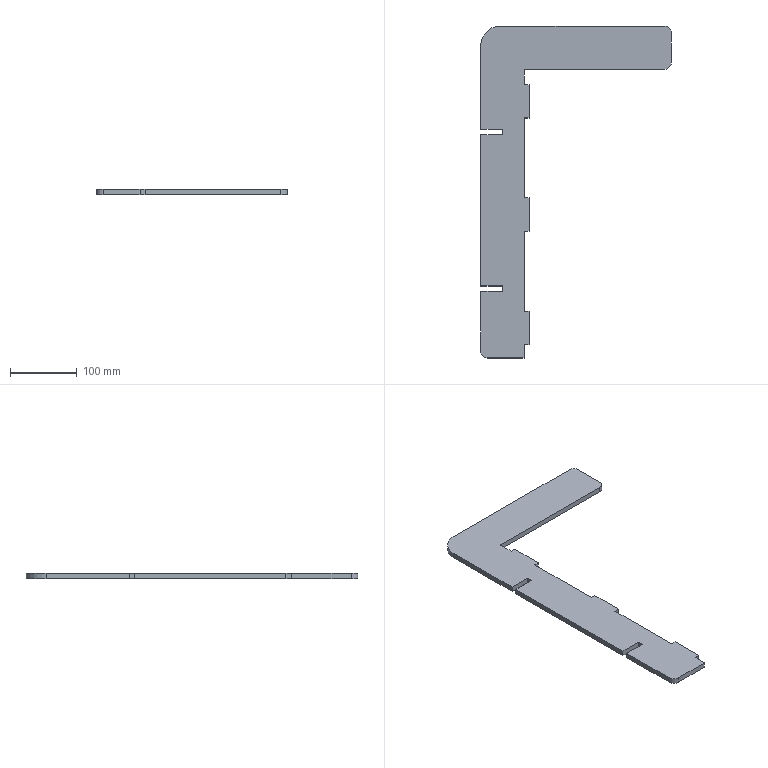Part | SolidWorks | features FlatPattern 1, SMBaseFlange 1, SheetMetal 1 | 1 solid | 33 faces | box 286 x 498 x 8 mm | volume 376603 mm3 | plane 28 | cylinder 5 | commonest cylinder face diameters 20 x3 4 x1 60 x1
STEP:
#1=CARTESIAN_POINT('',(350.505,-222.753,0.));
#2=VERTEX_POINT('',#1);
#3=CARTESIAN_POINT('',(350.505,-202.753,0.));
#4=VERTEX_POINT('',#3);
#5=CARTESIAN_POINT('',(350.505,-222.753,0.));
#6=DIRECTION('',(0.,1.,0.));
#7=VECTOR('',#6,1000.);
#8=LINE('',#5,#7);
#9=EDGE_CURVE('',#2,#4,#8,.T.);
#10=ORIENTED_EDGE('',*,*,#9,.F.);
#11=CARTESIAN_POINT('',(350.505,-222.753,-8.));
#12=VERTEX_POINT('',#11);
#13=CARTESIAN_POINT('',(350.505,-222.753,-8.));
#14=DIRECTION('',(0.,0.,1.));
#15=VECTOR('',#14,1000.);
#16=LINE('',#13,#15);
#17=EDGE_CURVE('',#12,#2,#16,.T.);
#18=ORIENTED_EDGE('',*,*,#17,.F.);
#19=CARTESIAN_POINT('',(350.505,-202.753,-8.));
#20=VERTEX_POINT('',#19);
#21=CARTESIAN_POINT('',(350.505,-222.753,-8.));
#22=DIRECTION('',(0.,1.,0.));
#23=VECTOR('',#22,1000.);
#24=LINE('',#21,#23);
#25=EDGE_CURVE('',#12,#20,#24,.T.);
#26=ORIENTED_EDGE('',*,*,#25,.T.);
#27=CARTESIAN_POINT('',(350.505,-202.753,-8.));
#28=DIRECTION('',(0.,0.,1.));
#29=VECTOR('',#28,1000.);
#30=LINE('',#27,#29);
#31=EDGE_CURVE('',#20,#4,#30,.T.);
#32=ORIENTED_EDGE('',*,*,#31,.T.);
#33=EDGE_LOOP('',(#10,#18,#26,#32));
#34=FACE_OUTER_BOUND('',#33,.T.);
#35=CARTESIAN_POINT('',(350.505,-222.753,-8.));
#36=DIRECTION('',(1.,0.,0.));
#37=DIRECTION('',(0.,0.,-1.));
#38=AXIS2_PLACEMENT_3D('',#35,#36,#37);
#39=PLANE('',#38);
#40=ADVANCED_FACE('',(#34),#39,.T.);
#41=CARTESIAN_POINT('',(295.505,-222.753,0.));
#42=VERTEX_POINT('',#41);
#43=CARTESIAN_POINT('',(295.505,-222.753,0.));
#44=DIRECTION('',(1.,0.,0.));
#45=VECTOR('',#44,1000.);
#46=LINE('',#43,#45);
#47=EDGE_CURVE('',#42,#2,#46,.T.);
#48=ORIENTED_EDGE('',*,*,#47,.F.);
#49=CARTESIAN_POINT('',(295.505,-222.753,-8.));
#50=VERTEX_POINT('',#49);
#51=CARTESIAN_POINT('',(295.505,-222.753,-8.));
#52=DIRECTION('',(0.,0.,1.));
#53=VECTOR('',#52,1000.);
#54=LINE('',#51,#53);
#55=EDGE_CURVE('',#50,#42,#54,.T.);
#56=ORIENTED_EDGE('',*,*,#55,.F.);
#57=CARTESIAN_POINT('',(295.505,-222.753,-8.));
#58=DIRECTION('',(1.,0.,0.));
#59=VECTOR('',#58,1000.);
#60=LINE('',#57,#59);
#61=EDGE_CURVE('',#50,#12,#60,.T.);
#62=ORIENTED_EDGE('',*,*,#61,.T.);
#63=ORIENTED_EDGE('',*,*,#17,.T.);
#64=EDGE_LOOP('',(#48,#56,#62,#63));
#65=FACE_OUTER_BOUND('',#64,.T.);
#66=CARTESIAN_POINT('',(295.505,-222.753,-8.));
#67=DIRECTION('',(0.,-1.,0.));
#68=DIRECTION('',(0.,0.,-1.));
#69=AXIS2_PLACEMENT_3D('',#66,#67,#68);
#70=PLANE('',#69);
#71=ADVANCED_FACE('',(#65),#70,.T.);
#72=CARTESIAN_POINT('',(285.505,-212.753,0.));
#73=VERTEX_POINT('',#72);
#74=CARTESIAN_POINT('',(295.505,-212.753,0.));
#75=DIRECTION('',(0.,0.,1.));
#76=DIRECTION('',(1.,0.,0.));
#77=AXIS2_PLACEMENT_3D('',#74,#75,#76);
#78=CIRCLE('',#77,10.);
#79=EDGE_CURVE('',#73,#42,#78,.T.);
#80=ORIENTED_EDGE('',*,*,#79,.F.);
#81=CARTESIAN_POINT('',(285.505,-212.753,-8.));
#82=VERTEX_POINT('',#81);
#83=CARTESIAN_POINT('',(285.505,-212.753,-8.));
#84=DIRECTION('',(0.,0.,1.));
#85=VECTOR('',#84,1000.);
#86=LINE('',#83,#85);
#87=EDGE_CURVE('',#82,#73,#86,.T.);
#88=ORIENTED_EDGE('',*,*,#87,.F.);
#89=CARTESIAN_POINT('',(295.505,-212.753,-8.));
#90=DIRECTION('',(0.,0.,1.));
#91=DIRECTION('',(1.,0.,0.));
#92=AXIS2_PLACEMENT_3D('',#89,#90,#91);
#93=CIRCLE('',#92,10.);
#94=EDGE_CURVE('',#82,#50,#93,.T.);
#95=ORIENTED_EDGE('',*,*,#94,.T.);
#96=ORIENTED_EDGE('',*,*,#55,.T.);
#97=EDGE_LOOP('',(#80,#88,#95,#96));
#98=FACE_OUTER_BOUND('',#97,.T.);
#99=CARTESIAN_POINT('',(295.505,-212.753,-8.));
#100=DIRECTION('',(0.,0.,1.));
#101=DIRECTION('',(1.,0.,0.));
#102=AXIS2_PLACEMENT_3D('',#99,#100,#101);
#103=CYLINDRICAL_SURFACE('',#102,10.);
#104=ADVANCED_FACE('',(#98),#103,.T.);
#105=CARTESIAN_POINT('',(285.505,-122.753,0.));
#106=VERTEX_POINT('',#105);
#107=CARTESIAN_POINT('',(285.505,-122.753,0.));
#108=DIRECTION('',(0.,-1.,0.));
#109=VECTOR('',#108,1000.);
#110=LINE('',#107,#109);
#111=EDGE_CURVE('',#106,#73,#110,.T.);
#112=ORIENTED_EDGE('',*,*,#111,.F.);
#113=CARTESIAN_POINT('',(285.505,-122.753,-8.));
#114=VERTEX_POINT('',#113);
#115=CARTESIAN_POINT('',(285.505,-122.753,-8.));
#116=DIRECTION('',(0.,0.,1.));
#117=VECTOR('',#116,1000.);
#118=LINE('',#115,#117);
#119=EDGE_CURVE('',#114,#106,#118,.T.);
#120=ORIENTED_EDGE('',*,*,#119,.F.);
#121=CARTESIAN_POINT('',(285.505,-122.753,-8.));
#122=DIRECTION('',(0.,-1.,0.));
#123=VECTOR('',#122,1000.);
#124=LINE('',#121,#123);
#125=EDGE_CURVE('',#114,#82,#124,.T.);
#126=ORIENTED_EDGE('',*,*,#125,.T.);
#127=ORIENTED_EDGE('',*,*,#87,.T.);
#128=EDGE_LOOP('',(#112,#120,#126,#127));
#129=FACE_OUTER_BOUND('',#128,.T.);
#130=CARTESIAN_POINT('',(285.505,-122.753,-8.));
#131=DIRECTION('',(-1.,0.,0.));
#132=DIRECTION('',(0.,-1.,0.));
#133=AXIS2_PLACEMENT_3D('',#130,#131,#132);
#134=PLANE('',#133);
#135=ADVANCED_FACE('',(#129),#134,.T.);
#136=CARTESIAN_POINT('',(318.505,-122.753,0.));
#137=VERTEX_POINT('',#136);
#138=CARTESIAN_POINT('',(318.505,-122.753,0.));
#139=DIRECTION('',(-1.,0.,0.));
#140=VECTOR('',#139,1000.);
#141=LINE('',#138,#140);
#142=EDGE_CURVE('',#137,#106,#141,.T.);
#143=ORIENTED_EDGE('',*,*,#142,.F.);
#144=CARTESIAN_POINT('',(318.505,-122.753,-8.));
#145=VERTEX_POINT('',#144);
#146=CARTESIAN_POINT('',(318.505,-122.753,-8.));
#147=DIRECTION('',(0.,0.,1.));
#148=VECTOR('',#147,1000.);
#149=LINE('',#146,#148);
#150=EDGE_CURVE('',#145,#137,#149,.T.);
#151=ORIENTED_EDGE('',*,*,#150,.F.);
#152=CARTESIAN_POINT('',(318.505,-122.753,-8.));
#153=DIRECTION('',(-1.,0.,0.));
#154=VECTOR('',#153,1000.);
#155=LINE('',#152,#154);
#156=EDGE_CURVE('',#145,#114,#155,.T.);
#157=ORIENTED_EDGE('',*,*,#156,.T.);
#158=ORIENTED_EDGE('',*,*,#119,.T.);
#159=EDGE_LOOP('',(#143,#151,#157,#158));
#160=FACE_OUTER_BOUND('',#159,.T.);
#161=CARTESIAN_POINT('',(318.505,-122.753,-8.));
#162=DIRECTION('',(0.,1.,0.));
#163=DIRECTION('',(-1.,0.,0.));
#164=AXIS2_PLACEMENT_3D('',#161,#162,#163);
#165=PLANE('',#164);
#166=ADVANCED_FACE('',(#160),#165,.T.);
#167=CARTESIAN_POINT('',(318.505,-114.753,0.));
#168=VERTEX_POINT('',#167);
#169=CARTESIAN_POINT('',(318.505,-114.753,0.));
#170=DIRECTION('',(0.,-1.,0.));
#171=VECTOR('',#170,1000.);
#172=LINE('',#169,#171);
#173=EDGE_CURVE('',#168,#137,#172,.T.);
#174=ORIENTED_EDGE('',*,*,#173,.F.);
#175=CARTESIAN_POINT('',(318.505,-114.753,-8.));
#176=VERTEX_POINT('',#175);
#177=CARTESIAN_POINT('',(318.505,-114.753,-8.));
#178=DIRECTION('',(0.,0.,1.));
#179=VECTOR('',#178,1000.);
#180=LINE('',#177,#179);
#181=EDGE_CURVE('',#176,#168,#180,.T.);
#182=ORIENTED_EDGE('',*,*,#181,.F.);
#183=CARTESIAN_POINT('',(318.505,-114.753,-8.));
#184=DIRECTION('',(0.,-1.,0.));
#185=VECTOR('',#184,1000.);
#186=LINE('',#183,#185);
#187=EDGE_CURVE('',#176,#145,#186,.T.);
#188=ORIENTED_EDGE('',*,*,#187,.T.);
#189=ORIENTED_EDGE('',*,*,#150,.T.);
#190=EDGE_LOOP('',(#174,#182,#188,#189));
#191=FACE_OUTER_BOUND('',#190,.T.);
#192=CARTESIAN_POINT('',(318.505,-114.753,-8.));
#193=DIRECTION('',(-1.,0.,0.));
#194=DIRECTION('',(0.,0.,1.));
#195=AXIS2_PLACEMENT_3D('',#192,#193,#194);
#196=PLANE('',#195);
#197=ADVANCED_FACE('',(#191),#196,.T.);
#198=CARTESIAN_POINT('',(285.505,-114.753,0.));
#199=VERTEX_POINT('',#198);
#200=CARTESIAN_POINT('',(285.505,-114.753,0.));
#201=DIRECTION('',(1.,0.,0.));
#202=VECTOR('',#201,1000.);
#203=LINE('',#200,#202);
#204=EDGE_CURVE('',#199,#168,#203,.T.);
#205=ORIENTED_EDGE('',*,*,#204,.F.);
#206=CARTESIAN_POINT('',(285.505,-114.753,-8.));
#207=VERTEX_POINT('',#206);
#208=CARTESIAN_POINT('',(285.505,-114.753,-8.));
#209=DIRECTION('',(0.,0.,1.));
#210=VECTOR('',#209,1000.);
#211=LINE('',#208,#210);
#212=EDGE_CURVE('',#207,#199,#211,.T.);
#213=ORIENTED_EDGE('',*,*,#212,.F.);
#214=CARTESIAN_POINT('',(285.505,-114.753,-8.));
#215=DIRECTION('',(1.,0.,0.));
#216=VECTOR('',#215,1000.);
#217=LINE('',#214,#216);
#218=EDGE_CURVE('',#207,#176,#217,.T.);
#219=ORIENTED_EDGE('',*,*,#218,.T.);
#220=ORIENTED_EDGE('',*,*,#181,.T.);
#221=EDGE_LOOP('',(#205,#213,#219,#220));
#222=FACE_OUTER_BOUND('',#221,.T.);
#223=CARTESIAN_POINT('',(285.505,-114.753,-8.));
#224=DIRECTION('',(0.,-1.,0.));
#225=DIRECTION('',(1.,0.,0.));
#226=AXIS2_PLACEMENT_3D('',#223,#224,#225);
#227=PLANE('',#226);
#228=ADVANCED_FACE('',(#222),#227,.T.);
#229=CARTESIAN_POINT('',(285.505,112.247,0.));
#230=VERTEX_POINT('',#229);
#231=CARTESIAN_POINT('',(285.505,112.247,0.));
#232=DIRECTION('',(0.,-1.,0.));
#233=VECTOR('',#232,1000.);
#234=LINE('',#231,#233);
#235=EDGE_CURVE('',#230,#199,#234,.T.);
#236=ORIENTED_EDGE('',*,*,#235,.F.);
#237=CARTESIAN_POINT('',(285.505,112.247,-8.));
#238=VERTEX_POINT('',#237);
#239=CARTESIAN_POINT('',(285.505,112.247,-8.));
#240=DIRECTION('',(0.,0.,1.));
#241=VECTOR('',#240,1000.);
#242=LINE('',#239,#241);
#243=EDGE_CURVE('',#238,#230,#242,.T.);
#244=ORIENTED_EDGE('',*,*,#243,.F.);
#245=CARTESIAN_POINT('',(285.505,112.247,-8.));
#246=DIRECTION('',(0.,-1.,0.));
#247=VECTOR('',#246,1000.);
#248=LINE('',#245,#247);
#249=EDGE_CURVE('',#238,#207,#248,.T.);
#250=ORIENTED_EDGE('',*,*,#249,.T.);
#251=ORIENTED_EDGE('',*,*,#212,.T.);
#252=EDGE_LOOP('',(#236,#244,#250,#251));
#253=FACE_OUTER_BOUND('',#252,.T.);
#254=CARTESIAN_POINT('',(285.505,112.247,-8.));
#255=DIRECTION('',(-1.,0.,0.));
#256=DIRECTION('',(0.,-1.,0.));
#257=AXIS2_PLACEMENT_3D('',#254,#255,#256);
#258=PLANE('',#257);
#259=ADVANCED_FACE('',(#253),#258,.T.);
#260=CARTESIAN_POINT('',(318.505,112.247,0.));
#261=VERTEX_POINT('',#260);
#262=CARTESIAN_POINT('',(318.505,112.247,0.));
#263=DIRECTION('',(-1.,0.,0.));
#264=VECTOR('',#263,1000.);
#265=LINE('',#262,#264);
#266=EDGE_CURVE('',#261,#230,#265,.T.);
#267=ORIENTED_EDGE('',*,*,#266,.F.);
#268=CARTESIAN_POINT('',(318.505,112.247,-8.));
#269=VERTEX_POINT('',#268);
#270=CARTESIAN_POINT('',(318.505,112.247,-8.));
#271=DIRECTION('',(0.,0.,1.));
#272=VECTOR('',#271,1000.);
#273=LINE('',#270,#272);
#274=EDGE_CURVE('',#269,#261,#273,.T.);
#275=ORIENTED_EDGE('',*,*,#274,.F.);
#276=CARTESIAN_POINT('',(318.505,112.247,-8.));
#277=DIRECTION('',(-1.,0.,0.));
#278=VECTOR('',#277,1000.);
#279=LINE('',#276,#278);
#280=EDGE_CURVE('',#269,#238,#279,.T.);
#281=ORIENTED_EDGE('',*,*,#280,.T.);
#282=ORIENTED_EDGE('',*,*,#243,.T.);
#283=EDGE_LOOP('',(#267,#275,#281,#282));
#284=FACE_OUTER_BOUND('',#283,.T.);
#285=CARTESIAN_POINT('',(318.505,112.247,-8.));
#286=DIRECTION('',(0.,1.,0.));
#287=DIRECTION('',(-1.,0.,0.));
#288=AXIS2_PLACEMENT_3D('',#285,#286,#287);
#289=PLANE('',#288);
#290=ADVANCED_FACE('',(#284),#289,.T.);
#291=CARTESIAN_POINT('',(318.505,120.247,0.));
#292=VERTEX_POINT('',#291);
#293=CARTESIAN_POINT('',(318.505,120.247,0.));
#294=DIRECTION('',(0.,-1.,0.));
#295=VECTOR('',#294,1000.);
#296=LINE('',#293,#295);
#297=EDGE_CURVE('',#292,#261,#296,.T.);
#298=ORIENTED_EDGE('',*,*,#297,.F.);
#299=CARTESIAN_POINT('',(318.505,120.247,-8.));
#300=VERTEX_POINT('',#299);
#301=CARTESIAN_POINT('',(318.505,120.247,-8.));
#302=DIRECTION('',(0.,0.,1.));
#303=VECTOR('',#302,1000.);
#304=LINE('',#301,#303);
#305=EDGE_CURVE('',#300,#292,#304,.T.);
#306=ORIENTED_EDGE('',*,*,#305,.F.);
#307=CARTESIAN_POINT('',(318.505,120.247,-8.));
#308=DIRECTION('',(0.,-1.,0.));
#309=VECTOR('',#308,1000.);
#310=LINE('',#307,#309);
#311=EDGE_CURVE('',#300,#269,#310,.T.);
#312=ORIENTED_EDGE('',*,*,#311,.T.);
#313=ORIENTED_EDGE('',*,*,#274,.T.);
#314=EDGE_LOOP('',(#298,#306,#312,#313));
#315=FACE_OUTER_BOUND('',#314,.T.);
#316=CARTESIAN_POINT('',(318.505,120.247,-8.));
#317=DIRECTION('',(-1.,0.,0.));
#318=DIRECTION('',(0.,0.,1.));
#319=AXIS2_PLACEMENT_3D('',#316,#317,#318);
#320=PLANE('',#319);
#321=ADVANCED_FACE('',(#315),#320,.T.);
#322=CARTESIAN_POINT('',(285.505,120.247,0.));
#323=VERTEX_POINT('',#322);
#324=CARTESIAN_POINT('',(318.505,120.247,0.));
#325=DIRECTION('',(1.,0.,0.));
#326=VECTOR('',#325,1000.);
#327=LINE('',#324,#326);
#328=EDGE_CURVE('',#323,#292,#327,.T.);
#329=ORIENTED_EDGE('',*,*,#328,.F.);
#330=CARTESIAN_POINT('',(285.505,120.247,-8.));
#331=VERTEX_POINT('',#330);
#332=CARTESIAN_POINT('',(285.505,120.247,-8.));
#333=DIRECTION('',(0.,0.,1.));
#334=VECTOR('',#333,1000.);
#335=LINE('',#332,#334);
#336=EDGE_CURVE('',#331,#323,#335,.T.);
#337=ORIENTED_EDGE('',*,*,#336,.F.);
#338=CARTESIAN_POINT('',(318.505,120.247,-8.));
#339=DIRECTION('',(1.,0.,0.));
#340=VECTOR('',#339,1000.);
#341=LINE('',#338,#340);
#342=EDGE_CURVE('',#331,#300,#341,.T.);
#343=ORIENTED_EDGE('',*,*,#342,.T.);
#344=ORIENTED_EDGE('',*,*,#305,.T.);
#345=EDGE_LOOP('',(#329,#337,#343,#344));
#346=FACE_OUTER_BOUND('',#345,.T.);
#347=CARTESIAN_POINT('',(318.505,120.247,-8.));
#348=DIRECTION('',(0.,-1.,0.));
#349=DIRECTION('',(1.,0.,0.));
#350=AXIS2_PLACEMENT_3D('',#347,#348,#349);
#351=PLANE('',#350);
#352=ADVANCED_FACE('',(#346),#351,.T.);
#353=CARTESIAN_POINT('',(285.505,245.247,0.));
#354=VERTEX_POINT('',#353);
#355=CARTESIAN_POINT('',(285.505,245.247,0.));
#356=DIRECTION('',(0.,-1.,0.));
#357=VECTOR('',#356,1000.);
#358=LINE('',#355,#357);
#359=EDGE_CURVE('',#354,#323,#358,.T.);
#360=ORIENTED_EDGE('',*,*,#359,.F.);
#361=CARTESIAN_POINT('',(285.505,245.247,-8.));
#362=VERTEX_POINT('',#361);
#363=CARTESIAN_POINT('',(285.505,245.247,-8.));
#364=DIRECTION('',(0.,0.,1.));
#365=VECTOR('',#364,1000.);
#366=LINE('',#363,#365);
#367=EDGE_CURVE('',#362,#354,#366,.T.);
#368=ORIENTED_EDGE('',*,*,#367,.F.);
#369=CARTESIAN_POINT('',(285.505,245.247,-8.));
#370=DIRECTION('',(0.,-1.,0.));
#371=VECTOR('',#370,1000.);
#372=LINE('',#369,#371);
#373=EDGE_CURVE('',#362,#331,#372,.T.);
#374=ORIENTED_EDGE('',*,*,#373,.T.);
#375=ORIENTED_EDGE('',*,*,#336,.T.);
#376=EDGE_LOOP('',(#360,#368,#374,#375));
#377=FACE_OUTER_BOUND('',#376,.T.);
#378=CARTESIAN_POINT('',(285.505,245.247,-8.));
#379=DIRECTION('',(-1.,0.,0.));
#380=DIRECTION('',(0.,-1.,0.));
#381=AXIS2_PLACEMENT_3D('',#378,#379,#380);
#382=PLANE('',#381);
#383=ADVANCED_FACE('',(#377),#382,.T.);
#384=CARTESIAN_POINT('',(315.505,275.247,0.));
#385=VERTEX_POINT('',#384);
#386=CARTESIAN_POINT('',(315.505,245.247,0.));
#387=DIRECTION('',(0.,0.,1.));
#388=DIRECTION('',(1.,0.,0.));
#389=AXIS2_PLACEMENT_3D('',#386,#387,#388);
#390=CIRCLE('',#389,30.);
#391=EDGE_CURVE('',#385,#354,#390,.T.);
#392=ORIENTED_EDGE('',*,*,#391,.F.);
#393=CARTESIAN_POINT('',(315.505,275.247,-8.));
#394=VERTEX_POINT('',#393);
#395=CARTESIAN_POINT('',(315.505,275.247,-8.));
#396=DIRECTION('',(0.,0.,1.));
#397=VECTOR('',#396,1000.);
#398=LINE('',#395,#397);
#399=EDGE_CURVE('',#394,#385,#398,.T.);
#400=ORIENTED_EDGE('',*,*,#399,.F.);
#401=CARTESIAN_POINT('',(315.505,245.247,-8.));
#402=DIRECTION('',(0.,0.,1.));
#403=DIRECTION('',(1.,0.,0.));
#404=AXIS2_PLACEMENT_3D('',#401,#402,#403);
#405=CIRCLE('',#404,30.);
#406=EDGE_CURVE('',#394,#362,#405,.T.);
#407=ORIENTED_EDGE('',*,*,#406,.T.);
#408=ORIENTED_EDGE('',*,*,#367,.T.);
#409=EDGE_LOOP('',(#392,#400,#407,#408));
#410=FACE_OUTER_BOUND('',#409,.T.);
#411=CARTESIAN_POINT('',(315.505,245.247,-8.));
#412=DIRECTION('',(0.,0.,1.));
#413=DIRECTION('',(1.,0.,0.));
#414=AXIS2_PLACEMENT_3D('',#411,#412,#413);
#415=CYLINDRICAL_SURFACE('',#414,30.);
#416=ADVANCED_FACE('',(#410),#415,.T.);
#417=CARTESIAN_POINT('',(561.505,275.247,0.));
#418=VERTEX_POINT('',#417);
#419=CARTESIAN_POINT('',(561.505,275.247,0.));
#420=DIRECTION('',(-1.,0.,0.));
#421=VECTOR('',#420,1000.);
#422=LINE('',#419,#421);
#423=EDGE_CURVE('',#418,#385,#422,.T.);
#424=ORIENTED_EDGE('',*,*,#423,.F.);
#425=CARTESIAN_POINT('',(561.505,275.247,-8.));
#426=VERTEX_POINT('',#425);
#427=CARTESIAN_POINT('',(561.505,275.247,-8.));
#428=DIRECTION('',(0.,0.,1.));
#429=VECTOR('',#428,1000.);
#430=LINE('',#427,#429);
#431=EDGE_CURVE('',#426,#418,#430,.T.);
#432=ORIENTED_EDGE('',*,*,#431,.F.);
#433=CARTESIAN_POINT('',(561.505,275.247,-8.));
#434=DIRECTION('',(-1.,0.,0.));
#435=VECTOR('',#434,1000.);
#436=LINE('',#433,#435);
#437=EDGE_CURVE('',#426,#394,#436,.T.);
#438=ORIENTED_EDGE('',*,*,#437,.T.);
#439=ORIENTED_EDGE('',*,*,#399,.T.);
#440=EDGE_LOOP('',(#424,#432,#438,#439));
#441=FACE_OUTER_BOUND('',#440,.T.);
#442=CARTESIAN_POINT('',(561.505,275.247,-8.));
#443=DIRECTION('',(0.,1.,0.));
#444=DIRECTION('',(-1.,0.,0.));
#445=AXIS2_PLACEMENT_3D('',#442,#443,#444);
#446=PLANE('',#445);
#447=ADVANCED_FACE('',(#441),#446,.T.);
#448=CARTESIAN_POINT('',(571.505,265.247,0.));
#449=VERTEX_POINT('',#448);
#450=CARTESIAN_POINT('',(561.505,265.247,0.));
#451=DIRECTION('',(0.,0.,1.));
#452=DIRECTION('',(1.,0.,0.));
#453=AXIS2_PLACEMENT_3D('',#450,#451,#452);
#454=CIRCLE('',#453,10.);
#455=EDGE_CURVE('',#449,#418,#454,.T.);
#456=ORIENTED_EDGE('',*,*,#455,.F.);
#457=CARTESIAN_POINT('',(571.505,265.247,-8.));
#458=VERTEX_POINT('',#457);
#459=CARTESIAN_POINT('',(571.505,265.247,-8.));
#460=DIRECTION('',(0.,0.,1.));
#461=VECTOR('',#460,1000.);
#462=LINE('',#459,#461);
#463=EDGE_CURVE('',#458,#449,#462,.T.);
#464=ORIENTED_EDGE('',*,*,#463,.F.);
#465=CARTESIAN_POINT('',(561.505,265.247,-8.));
#466=DIRECTION('',(0.,0.,1.));
#467=DIRECTION('',(1.,0.,0.));
#468=AXIS2_PLACEMENT_3D('',#465,#466,#467);
#469=CIRCLE('',#468,10.);
#470=EDGE_CURVE('',#458,#426,#469,.T.);
#471=ORIENTED_EDGE('',*,*,#470,.T.);
#472=ORIENTED_EDGE('',*,*,#431,.T.);
#473=EDGE_LOOP('',(#456,#464,#471,#472));
#474=FACE_OUTER_BOUND('',#473,.T.);
#475=CARTESIAN_POINT('',(561.505,265.247,-8.));
#476=DIRECTION('',(0.,0.,1.));
#477=DIRECTION('',(1.,0.,0.));
#478=AXIS2_PLACEMENT_3D('',#475,#476,#477);
#479=CYLINDRICAL_SURFACE('',#478,10.);
#480=ADVANCED_FACE('',(#474),#479,.T.);
#481=CARTESIAN_POINT('',(571.505,220.247,0.));
#482=VERTEX_POINT('',#481);
#483=CARTESIAN_POINT('',(571.505,220.247,0.));
#484=DIRECTION('',(0.,1.,0.));
#485=VECTOR('',#484,1000.);
#486=LINE('',#483,#485);
#487=EDGE_CURVE('',#482,#449,#486,.T.);
#488=ORIENTED_EDGE('',*,*,#487,.F.);
#489=CARTESIAN_POINT('',(571.505,220.247,-8.));
#490=VERTEX_POINT('',#489);
#491=CARTESIAN_POINT('',(571.505,220.247,-8.));
#492=DIRECTION('',(0.,0.,1.));
#493=VECTOR('',#492,1000.);
#494=LINE('',#491,#493);
#495=EDGE_CURVE('',#490,#482,#494,.T.);
#496=ORIENTED_EDGE('',*,*,#495,.F.);
#497=CARTESIAN_POINT('',(571.505,220.247,-8.));
#498=DIRECTION('',(0.,1.,0.));
#499=VECTOR('',#498,1000.);
#500=LINE('',#497,#499);
#501=EDGE_CURVE('',#490,#458,#500,.T.);
#502=ORIENTED_EDGE('',*,*,#501,.T.);
#503=ORIENTED_EDGE('',*,*,#463,.T.);
#504=EDGE_LOOP('',(#488,#496,#502,#503));
#505=FACE_OUTER_BOUND('',#504,.T.);
#506=CARTESIAN_POINT('',(571.505,220.247,-8.));
#507=DIRECTION('',(1.,0.,0.));
#508=DIRECTION('',(0.,1.,0.));
#509=AXIS2_PLACEMENT_3D('',#506,#507,#508);
#510=PLANE('',#509);
#511=ADVANCED_FACE('',(#505),#510,.T.);
#512=CARTESIAN_POINT('',(561.505,210.247,0.));
#513=VERTEX_POINT('',#512);
#514=CARTESIAN_POINT('',(561.505,220.247,0.));
#515=DIRECTION('',(0.,0.,1.));
#516=DIRECTION('',(1.,0.,0.));
#517=AXIS2_PLACEMENT_3D('',#514,#515,#516);
#518=CIRCLE('',#517,10.);
#519=EDGE_CURVE('',#513,#482,#518,.T.);
#520=ORIENTED_EDGE('',*,*,#519,.F.);
#521=CARTESIAN_POINT('',(561.505,210.247,-8.));
#522=VERTEX_POINT('',#521);
#523=CARTESIAN_POINT('',(561.505,210.247,-8.));
#524=DIRECTION('',(0.,0.,1.));
#525=VECTOR('',#524,1000.);
#526=LINE('',#523,#525);
#527=EDGE_CURVE('',#522,#513,#526,.T.);
#528=ORIENTED_EDGE('',*,*,#527,.F.);
#529=CARTESIAN_POINT('',(561.505,220.247,-8.));
#530=DIRECTION('',(0.,0.,1.));
#531=DIRECTION('',(1.,0.,0.));
#532=AXIS2_PLACEMENT_3D('',#529,#530,#531);
#533=CIRCLE('',#532,10.);
#534=EDGE_CURVE('',#522,#490,#533,.T.);
#535=ORIENTED_EDGE('',*,*,#534,.T.);
#536=ORIENTED_EDGE('',*,*,#495,.T.);
#537=EDGE_LOOP('',(#520,#528,#535,#536));
#538=FACE_OUTER_BOUND('',#537,.T.);
#539=CARTESIAN_POINT('',(561.505,220.247,-8.));
#540=DIRECTION('',(0.,0.,1.));
#541=DIRECTION('',(1.,0.,0.));
#542=AXIS2_PLACEMENT_3D('',#539,#540,#541);
#543=CYLINDRICAL_SURFACE('',#542,10.);
#544=ADVANCED_FACE('',(#538),#543,.T.);
#545=CARTESIAN_POINT('',(352.505,210.247,0.));
#546=VERTEX_POINT('',#545);
#547=CARTESIAN_POINT('',(352.505,210.247,0.));
#548=DIRECTION('',(1.,0.,0.));
#549=VECTOR('',#548,1000.);
#550=LINE('',#547,#549);
#551=EDGE_CURVE('',#546,#513,#550,.T.);
#552=ORIENTED_EDGE('',*,*,#551,.F.);
#553=CARTESIAN_POINT('',(352.505,210.247,-8.));
#554=VERTEX_POINT('',#553);
#555=CARTESIAN_POINT('',(352.505,210.247,-8.));
#556=DIRECTION('',(0.,0.,1.));
#557=VECTOR('',#556,1000.);
#558=LINE('',#555,#557);
#559=EDGE_CURVE('',#554,#546,#558,.T.);
#560=ORIENTED_EDGE('',*,*,#559,.F.);
#561=CARTESIAN_POINT('',(352.505,210.247,-8.));
#562=DIRECTION('',(1.,0.,0.));
#563=VECTOR('',#562,1000.);
#564=LINE('',#561,#563);
#565=EDGE_CURVE('',#554,#522,#564,.T.);
#566=ORIENTED_EDGE('',*,*,#565,.T.);
#567=ORIENTED_EDGE('',*,*,#527,.T.);
#568=EDGE_LOOP('',(#552,#560,#566,#567));
#569=FACE_OUTER_BOUND('',#568,.T.);
#570=CARTESIAN_POINT('',(352.505,210.247,-8.));
#571=DIRECTION('',(0.,-1.,0.));
#572=DIRECTION('',(0.,0.,-1.));
#573=AXIS2_PLACEMENT_3D('',#570,#571,#572);
#574=PLANE('',#573);
#575=ADVANCED_FACE('',(#569),#574,.T.);
#576=CARTESIAN_POINT('',(350.505,208.247,0.));
#577=VERTEX_POINT('',#576);
#578=CARTESIAN_POINT('',(352.505,208.247,0.));
#579=DIRECTION('',(0.,0.,-1.));
#580=DIRECTION('',(-1.,0.,0.));
#581=AXIS2_PLACEMENT_3D('',#578,#579,#580);
#582=CIRCLE('',#581,2.);
#583=EDGE_CURVE('',#577,#546,#582,.T.);
#584=ORIENTED_EDGE('',*,*,#583,.F.);
#585=CARTESIAN_POINT('',(350.505,208.247,-8.));
#586=VERTEX_POINT('',#585);
#587=CARTESIAN_POINT('',(350.505,208.247,-8.));
#588=DIRECTION('',(0.,0.,1.));
#589=VECTOR('',#588,1000.);
#590=LINE('',#587,#589);
#591=EDGE_CURVE('',#586,#577,#590,.T.);
#592=ORIENTED_EDGE('',*,*,#591,.F.);
#593=CARTESIAN_POINT('',(352.505,208.247,-8.));
#594=DIRECTION('',(0.,0.,-1.));
#595=DIRECTION('',(-1.,0.,0.));
#596=AXIS2_PLACEMENT_3D('',#593,#594,#595);
#597=CIRCLE('',#596,2.);
#598=EDGE_CURVE('',#586,#554,#597,.T.);
#599=ORIENTED_EDGE('',*,*,#598,.T.);
#600=ORIENTED_EDGE('',*,*,#559,.T.);
#601=EDGE_LOOP('',(#584,#592,#599,#600));
#602=FACE_OUTER_BOUND('',#601,.T.);
#603=CARTESIAN_POINT('',(352.505,208.247,-8.));
#604=DIRECTION('',(0.,0.,1.));
#605=DIRECTION('',(1.,0.,0.));
#606=AXIS2_PLACEMENT_3D('',#603,#604,#605);
#607=CYLINDRICAL_SURFACE('',#606,2.);
#608=ADVANCED_FACE('',(#602),#607,.F.);
#609=CARTESIAN_POINT('',(350.505,187.247,0.));
#610=VERTEX_POINT('',#609);
#611=CARTESIAN_POINT('',(350.505,187.247,0.));
#612=DIRECTION('',(0.,1.,0.));
#613=VECTOR('',#612,1000.);
#614=LINE('',#611,#613);
#615=EDGE_CURVE('',#610,#577,#614,.T.);
#616=ORIENTED_EDGE('',*,*,#615,.F.);
#617=CARTESIAN_POINT('',(350.505,187.247,-8.));
#618=VERTEX_POINT('',#617);
#619=CARTESIAN_POINT('',(350.505,187.247,-8.));
#620=DIRECTION('',(0.,0.,1.));
#621=VECTOR('',#620,1000.);
#622=LINE('',#619,#621);
#623=EDGE_CURVE('',#618,#610,#622,.T.);
#624=ORIENTED_EDGE('',*,*,#623,.F.);
#625=CARTESIAN_POINT('',(350.505,187.247,-8.));
#626=DIRECTION('',(0.,1.,0.));
#627=VECTOR('',#626,1000.);
#628=LINE('',#625,#627);
#629=EDGE_CURVE('',#618,#586,#628,.T.);
#630=ORIENTED_EDGE('',*,*,#629,.T.);
#631=ORIENTED_EDGE('',*,*,#591,.T.);
#632=EDGE_LOOP('',(#616,#624,#630,#631));
#633=FACE_OUTER_BOUND('',#632,.T.);
#634=CARTESIAN_POINT('',(350.505,187.247,-8.));
#635=DIRECTION('',(1.,0.,0.));
#636=DIRECTION('',(0.,1.,0.));
#637=AXIS2_PLACEMENT_3D('',#634,#635,#636);
#638=PLANE('',#637);
#639=ADVANCED_FACE('',(#633),#638,.T.);
#640=CARTESIAN_POINT('',(358.005,187.247,0.));
#641=VERTEX_POINT('',#640);
#642=CARTESIAN_POINT('',(358.005,187.247,0.));
#643=DIRECTION('',(-1.,0.,0.));
#644=VECTOR('',#643,1000.);
#645=LINE('',#642,#644);
#646=EDGE_CURVE('',#641,#610,#645,.T.);
#647=ORIENTED_EDGE('',*,*,#646,.F.);
#648=CARTESIAN_POINT('',(358.005,187.247,-8.));
#649=VERTEX_POINT('',#648);
#650=CARTESIAN_POINT('',(358.005,187.247,-8.));
#651=DIRECTION('',(0.,0.,1.));
#652=VECTOR('',#651,1000.);
#653=LINE('',#650,#652);
#654=EDGE_CURVE('',#649,#641,#653,.T.);
#655=ORIENTED_EDGE('',*,*,#654,.F.);
#656=CARTESIAN_POINT('',(358.005,187.247,-8.));
#657=DIRECTION('',(-1.,0.,0.));
#658=VECTOR('',#657,1000.);
#659=LINE('',#656,#658);
#660=EDGE_CURVE('',#649,#618,#659,.T.);
#661=ORIENTED_EDGE('',*,*,#660,.T.);
#662=ORIENTED_EDGE('',*,*,#623,.T.);
#663=EDGE_LOOP('',(#647,#655,#661,#662));
#664=FACE_OUTER_BOUND('',#663,.T.);
#665=CARTESIAN_POINT('',(358.005,187.247,-8.));
#666=DIRECTION('',(0.,1.,0.));
#667=DIRECTION('',(0.,0.,1.));
#668=AXIS2_PLACEMENT_3D('',#665,#666,#667);
#669=PLANE('',#668);
#670=ADVANCED_FACE('',(#664),#669,.T.);
#671=CARTESIAN_POINT('',(358.005,137.247,0.));
#672=VERTEX_POINT('',#671);
#673=CARTESIAN_POINT('',(358.005,137.247,0.));
#674=DIRECTION('',(0.,1.,0.));
#675=VECTOR('',#674,1000.);
#676=LINE('',#673,#675);
#677=EDGE_CURVE('',#672,#641,#676,.T.);
#678=ORIENTED_EDGE('',*,*,#677,.F.);
#679=CARTESIAN_POINT('',(358.005,137.247,-8.));
#680=VERTEX_POINT('',#679);
#681=CARTESIAN_POINT('',(358.005,137.247,-8.));
#682=DIRECTION('',(0.,0.,1.));
#683=VECTOR('',#682,1000.);
#684=LINE('',#681,#683);
#685=EDGE_CURVE('',#680,#672,#684,.T.);
#686=ORIENTED_EDGE('',*,*,#685,.F.);
#687=CARTESIAN_POINT('',(358.005,137.247,-8.));
#688=DIRECTION('',(0.,1.,0.));
#689=VECTOR('',#688,1000.);
#690=LINE('',#687,#689);
#691=EDGE_CURVE('',#680,#649,#690,.T.);
#692=ORIENTED_EDGE('',*,*,#691,.T.);
#693=ORIENTED_EDGE('',*,*,#654,.T.);
#694=EDGE_LOOP('',(#678,#686,#692,#693));
#695=FACE_OUTER_BOUND('',#694,.T.);
#696=CARTESIAN_POINT('',(358.005,137.247,-8.));
#697=DIRECTION('',(1.,0.,0.));
#698=DIRECTION('',(0.,0.,-1.));
#699=AXIS2_PLACEMENT_3D('',#696,#697,#698);
#700=PLANE('',#699);
#701=ADVANCED_FACE('',(#695),#700,.T.);
#702=CARTESIAN_POINT('',(350.505,137.247,0.));
#703=VERTEX_POINT('',#702);
#704=CARTESIAN_POINT('',(350.505,137.247,0.));
#705=DIRECTION('',(1.,0.,0.));
#706=VECTOR('',#705,1000.);
#707=LINE('',#704,#706);
#708=EDGE_CURVE('',#703,#672,#707,.T.);
#709=ORIENTED_EDGE('',*,*,#708,.F.);
#710=CARTESIAN_POINT('',(350.505,137.247,-8.));
#711=VERTEX_POINT('',#710);
#712=CARTESIAN_POINT('',(350.505,137.247,-8.));
#713=DIRECTION('',(0.,0.,1.));
#714=VECTOR('',#713,1000.);
#715=LINE('',#712,#714);
#716=EDGE_CURVE('',#711,#703,#715,.T.);
#717=ORIENTED_EDGE('',*,*,#716,.F.);
#718=CARTESIAN_POINT('',(350.505,137.247,-8.));
#719=DIRECTION('',(1.,0.,0.));
#720=VECTOR('',#719,1000.);
#721=LINE('',#718,#720);
#722=EDGE_CURVE('',#711,#680,#721,.T.);
#723=ORIENTED_EDGE('',*,*,#722,.T.);
#724=ORIENTED_EDGE('',*,*,#685,.T.);
#725=EDGE_LOOP('',(#709,#717,#723,#724));
#726=FACE_OUTER_BOUND('',#725,.T.);
#727=CARTESIAN_POINT('',(350.505,137.247,-8.));
#728=DIRECTION('',(0.,-1.,0.));
#729=DIRECTION('',(0.,0.,-1.));
#730=AXIS2_PLACEMENT_3D('',#727,#728,#729);
#731=PLANE('',#730);
#732=ADVANCED_FACE('',(#726),#731,.T.);
#733=CARTESIAN_POINT('',(350.505,17.247,0.));
#734=VERTEX_POINT('',#733);
#735=CARTESIAN_POINT('',(350.505,17.247,0.));
#736=DIRECTION('',(0.,1.,0.));
#737=VECTOR('',#736,1000.);
#738=LINE('',#735,#737);
#739=EDGE_CURVE('',#734,#703,#738,.T.);
#740=ORIENTED_EDGE('',*,*,#739,.F.);
#741=CARTESIAN_POINT('',(350.505,17.247,-8.));
#742=VERTEX_POINT('',#741);
#743=CARTESIAN_POINT('',(350.505,17.247,-8.));
#744=DIRECTION('',(0.,0.,1.));
#745=VECTOR('',#744,1000.);
#746=LINE('',#743,#745);
#747=EDGE_CURVE('',#742,#734,#746,.T.);
#748=ORIENTED_EDGE('',*,*,#747,.F.);
#749=CARTESIAN_POINT('',(350.505,17.247,-8.));
#750=DIRECTION('',(0.,1.,0.));
#751=VECTOR('',#750,1000.);
#752=LINE('',#749,#751);
#753=EDGE_CURVE('',#742,#711,#752,.T.);
#754=ORIENTED_EDGE('',*,*,#753,.T.);
#755=ORIENTED_EDGE('',*,*,#716,.T.);
#756=EDGE_LOOP('',(#740,#748,#754,#755));
#757=FACE_OUTER_BOUND('',#756,.T.);
#758=CARTESIAN_POINT('',(350.505,17.247,-8.));
#759=DIRECTION('',(1.,0.,0.));
#760=DIRECTION('',(0.,0.,-1.));
#761=AXIS2_PLACEMENT_3D('',#758,#759,#760);
#762=PLANE('',#761);
#763=ADVANCED_FACE('',(#757),#762,.T.);
#764=CARTESIAN_POINT('',(358.005,17.247,0.));
#765=VERTEX_POINT('',#764);
#766=CARTESIAN_POINT('',(358.005,17.247,0.));
#767=DIRECTION('',(-1.,0.,0.));
#768=VECTOR('',#767,1000.);
#769=LINE('',#766,#768);
#770=EDGE_CURVE('',#765,#734,#769,.T.);
#771=ORIENTED_EDGE('',*,*,#770,.F.);
#772=CARTESIAN_POINT('',(358.005,17.247,-8.));
#773=VERTEX_POINT('',#772);
#774=CARTESIAN_POINT('',(358.005,17.247,-8.));
#775=DIRECTION('',(0.,0.,1.));
#776=VECTOR('',#775,1000.);
#777=LINE('',#774,#776);
#778=EDGE_CURVE('',#773,#765,#777,.T.);
#779=ORIENTED_EDGE('',*,*,#778,.F.);
#780=CARTESIAN_POINT('',(358.005,17.247,-8.));
#781=DIRECTION('',(-1.,0.,0.));
#782=VECTOR('',#781,1000.);
#783=LINE('',#780,#782);
#784=EDGE_CURVE('',#773,#742,#783,.T.);
#785=ORIENTED_EDGE('',*,*,#784,.T.);
#786=ORIENTED_EDGE('',*,*,#747,.T.);
#787=EDGE_LOOP('',(#771,#779,#785,#786));
#788=FACE_OUTER_BOUND('',#787,.T.);
#789=CARTESIAN_POINT('',(358.005,17.247,-8.));
#790=DIRECTION('',(0.,1.,0.));
#791=DIRECTION('',(0.,0.,1.));
#792=AXIS2_PLACEMENT_3D('',#789,#790,#791);
#793=PLANE('',#792);
#794=ADVANCED_FACE('',(#788),#793,.T.);
#795=CARTESIAN_POINT('',(358.005,-32.753,0.));
#796=VERTEX_POINT('',#795);
#797=CARTESIAN_POINT('',(358.005,-32.753,0.));
#798=DIRECTION('',(0.,1.,0.));
#799=VECTOR('',#798,1000.);
#800=LINE('',#797,#799);
#801=EDGE_CURVE('',#796,#765,#800,.T.);
#802=ORIENTED_EDGE('',*,*,#801,.F.);
#803=CARTESIAN_POINT('',(358.005,-32.753,-8.));
#804=VERTEX_POINT('',#803);
#805=CARTESIAN_POINT('',(358.005,-32.753,-8.));
#806=DIRECTION('',(0.,0.,1.));
#807=VECTOR('',#806,1000.);
#808=LINE('',#805,#807);
#809=EDGE_CURVE('',#804,#796,#808,.T.);
#810=ORIENTED_EDGE('',*,*,#809,.F.);
#811=CARTESIAN_POINT('',(358.005,-32.753,-8.));
#812=DIRECTION('',(0.,1.,0.));
#813=VECTOR('',#812,1000.);
#814=LINE('',#811,#813);
#815=EDGE_CURVE('',#804,#773,#814,.T.);
#816=ORIENTED_EDGE('',*,*,#815,.T.);
#817=ORIENTED_EDGE('',*,*,#778,.T.);
#818=EDGE_LOOP('',(#802,#810,#816,#817));
#819=FACE_OUTER_BOUND('',#818,.T.);
#820=CARTESIAN_POINT('',(358.005,-32.753,-8.));
#821=DIRECTION('',(1.,0.,0.));
#822=DIRECTION('',(0.,0.,-1.));
#823=AXIS2_PLACEMENT_3D('',#820,#821,#822);
#824=PLANE('',#823);
#825=ADVANCED_FACE('',(#819),#824,.T.);
#826=CARTESIAN_POINT('',(350.505,-32.753,0.));
#827=VERTEX_POINT('',#826);
#828=CARTESIAN_POINT('',(350.505,-32.753,0.));
#829=DIRECTION('',(1.,0.,0.));
#830=VECTOR('',#829,1000.);
#831=LINE('',#828,#830);
#832=EDGE_CURVE('',#827,#796,#831,.T.);
#833=ORIENTED_EDGE('',*,*,#832,.F.);
#834=CARTESIAN_POINT('',(350.505,-32.753,-8.));
#835=VERTEX_POINT('',#834);
#836=CARTESIAN_POINT('',(350.505,-32.753,-8.));
#837=DIRECTION('',(0.,0.,1.));
#838=VECTOR('',#837,1000.);
#839=LINE('',#836,#838);
#840=EDGE_CURVE('',#835,#827,#839,.T.);
#841=ORIENTED_EDGE('',*,*,#840,.F.);
#842=CARTESIAN_POINT('',(350.505,-32.753,-8.));
#843=DIRECTION('',(1.,0.,0.));
#844=VECTOR('',#843,1000.);
#845=LINE('',#842,#844);
#846=EDGE_CURVE('',#835,#804,#845,.T.);
#847=ORIENTED_EDGE('',*,*,#846,.T.);
#848=ORIENTED_EDGE('',*,*,#809,.T.);
#849=EDGE_LOOP('',(#833,#841,#847,#848));
#850=FACE_OUTER_BOUND('',#849,.T.);
#851=CARTESIAN_POINT('',(350.505,-32.753,-8.));
#852=DIRECTION('',(0.,-1.,0.));
#853=DIRECTION('',(0.,0.,-1.));
#854=AXIS2_PLACEMENT_3D('',#851,#852,#853);
#855=PLANE('',#854);
#856=ADVANCED_FACE('',(#850),#855,.T.);
#857=CARTESIAN_POINT('',(350.505,-152.753,0.));
#858=VERTEX_POINT('',#857);
#859=CARTESIAN_POINT('',(350.505,-152.753,0.));
#860=DIRECTION('',(0.,1.,0.));
#861=VECTOR('',#860,1000.);
#862=LINE('',#859,#861);
#863=EDGE_CURVE('',#858,#827,#862,.T.);
#864=ORIENTED_EDGE('',*,*,#863,.F.);
#865=CARTESIAN_POINT('',(350.505,-152.753,-8.));
#866=VERTEX_POINT('',#865);
#867=CARTESIAN_POINT('',(350.505,-152.753,-8.));
#868=DIRECTION('',(0.,0.,1.));
#869=VECTOR('',#868,1000.);
#870=LINE('',#867,#869);
#871=EDGE_CURVE('',#866,#858,#870,.T.);
#872=ORIENTED_EDGE('',*,*,#871,.F.);
#873=CARTESIAN_POINT('',(350.505,-152.753,-8.));
#874=DIRECTION('',(0.,1.,0.));
#875=VECTOR('',#874,1000.);
#876=LINE('',#873,#875);
#877=EDGE_CURVE('',#866,#835,#876,.T.);
#878=ORIENTED_EDGE('',*,*,#877,.T.);
#879=ORIENTED_EDGE('',*,*,#840,.T.);
#880=EDGE_LOOP('',(#864,#872,#878,#879));
#881=FACE_OUTER_BOUND('',#880,.T.);
#882=CARTESIAN_POINT('',(350.505,-152.753,-8.));
#883=DIRECTION('',(1.,0.,0.));
#884=DIRECTION('',(0.,0.,-1.));
#885=AXIS2_PLACEMENT_3D('',#882,#883,#884);
#886=PLANE('',#885);
#887=ADVANCED_FACE('',(#881),#886,.T.);
#888=CARTESIAN_POINT('',(358.005,-152.753,0.));
#889=VERTEX_POINT('',#888);
#890=CARTESIAN_POINT('',(358.005,-152.753,0.));
#891=DIRECTION('',(-1.,0.,0.));
#892=VECTOR('',#891,1000.);
#893=LINE('',#890,#892);
#894=EDGE_CURVE('',#889,#858,#893,.T.);
#895=ORIENTED_EDGE('',*,*,#894,.F.);
#896=CARTESIAN_POINT('',(358.005,-152.753,-8.));
#897=VERTEX_POINT('',#896);
#898=CARTESIAN_POINT('',(358.005,-152.753,-8.));
#899=DIRECTION('',(0.,0.,1.));
#900=VECTOR('',#899,1000.);
#901=LINE('',#898,#900);
#902=EDGE_CURVE('',#897,#889,#901,.T.);
#903=ORIENTED_EDGE('',*,*,#902,.F.);
#904=CARTESIAN_POINT('',(358.005,-152.753,-8.));
#905=DIRECTION('',(-1.,0.,0.));
#906=VECTOR('',#905,1000.);
#907=LINE('',#904,#906);
#908=EDGE_CURVE('',#897,#866,#907,.T.);
#909=ORIENTED_EDGE('',*,*,#908,.T.);
#910=ORIENTED_EDGE('',*,*,#871,.T.);
#911=EDGE_LOOP('',(#895,#903,#909,#910));
#912=FACE_OUTER_BOUND('',#911,.T.);
#913=CARTESIAN_POINT('',(358.005,-152.753,-8.));
#914=DIRECTION('',(0.,1.,0.));
#915=DIRECTION('',(0.,0.,1.));
#916=AXIS2_PLACEMENT_3D('',#913,#914,#915);
#917=PLANE('',#916);
#918=ADVANCED_FACE('',(#912),#917,.T.);
#919=CARTESIAN_POINT('',(358.005,-202.753,0.));
#920=VERTEX_POINT('',#919);
#921=CARTESIAN_POINT('',(358.005,-202.753,0.));
#922=DIRECTION('',(0.,1.,0.));
#923=VECTOR('',#922,1000.);
#924=LINE('',#921,#923);
#925=EDGE_CURVE('',#920,#889,#924,.T.);
#926=ORIENTED_EDGE('',*,*,#925,.F.);
#927=CARTESIAN_POINT('',(358.005,-202.753,-8.));
#928=VERTEX_POINT('',#927);
#929=CARTESIAN_POINT('',(358.005,-202.753,-8.));
#930=DIRECTION('',(0.,0.,1.));
#931=VECTOR('',#930,1000.);
#932=LINE('',#929,#931);
#933=EDGE_CURVE('',#928,#920,#932,.T.);
#934=ORIENTED_EDGE('',*,*,#933,.F.);
#935=CARTESIAN_POINT('',(358.005,-202.753,-8.));
#936=DIRECTION('',(0.,1.,0.));
#937=VECTOR('',#936,1000.);
#938=LINE('',#935,#937);
#939=EDGE_CURVE('',#928,#897,#938,.T.);
#940=ORIENTED_EDGE('',*,*,#939,.T.);
#941=ORIENTED_EDGE('',*,*,#902,.T.);
#942=EDGE_LOOP('',(#926,#934,#940,#941));
#943=FACE_OUTER_BOUND('',#942,.T.);
#944=CARTESIAN_POINT('',(358.005,-202.753,-8.));
#945=DIRECTION('',(1.,0.,0.));
#946=DIRECTION('',(0.,0.,-1.));
#947=AXIS2_PLACEMENT_3D('',#944,#945,#946);
#948=PLANE('',#947);
#949=ADVANCED_FACE('',(#943),#948,.T.);
#950=CARTESIAN_POINT('',(350.505,-202.753,0.));
#951=DIRECTION('',(1.,0.,0.));
#952=VECTOR('',#951,1000.);
#953=LINE('',#950,#952);
#954=EDGE_CURVE('',#4,#920,#953,.T.);
#955=ORIENTED_EDGE('',*,*,#954,.F.);
#956=ORIENTED_EDGE('',*,*,#31,.F.);
#957=CARTESIAN_POINT('',(350.505,-202.753,-8.));
#958=DIRECTION('',(1.,0.,0.));
#959=VECTOR('',#958,1000.);
#960=LINE('',#957,#959);
#961=EDGE_CURVE('',#20,#928,#960,.T.);
#962=ORIENTED_EDGE('',*,*,#961,.T.);
#963=ORIENTED_EDGE('',*,*,#933,.T.);
#964=EDGE_LOOP('',(#955,#956,#962,#963));
#965=FACE_OUTER_BOUND('',#964,.T.);
#966=CARTESIAN_POINT('',(350.505,-202.753,-8.));
#967=DIRECTION('',(0.,-1.,0.));
#968=DIRECTION('',(0.,0.,-1.));
#969=AXIS2_PLACEMENT_3D('',#966,#967,#968);
#970=PLANE('',#969);
#971=ADVANCED_FACE('',(#965),#970,.T.);
#972=ORIENTED_EDGE('',*,*,#25,.F.);
#973=ORIENTED_EDGE('',*,*,#61,.F.);
#974=ORIENTED_EDGE('',*,*,#94,.F.);
#975=ORIENTED_EDGE('',*,*,#125,.F.);
#976=ORIENTED_EDGE('',*,*,#156,.F.);
#977=ORIENTED_EDGE('',*,*,#187,.F.);
#978=ORIENTED_EDGE('',*,*,#218,.F.);
#979=ORIENTED_EDGE('',*,*,#249,.F.);
#980=ORIENTED_EDGE('',*,*,#280,.F.);
#981=ORIENTED_EDGE('',*,*,#311,.F.);
#982=ORIENTED_EDGE('',*,*,#342,.F.);
#983=ORIENTED_EDGE('',*,*,#373,.F.);
#984=ORIENTED_EDGE('',*,*,#406,.F.);
#985=ORIENTED_EDGE('',*,*,#437,.F.);
#986=ORIENTED_EDGE('',*,*,#470,.F.);
#987=ORIENTED_EDGE('',*,*,#501,.F.);
#988=ORIENTED_EDGE('',*,*,#534,.F.);
#989=ORIENTED_EDGE('',*,*,#565,.F.);
#990=ORIENTED_EDGE('',*,*,#598,.F.);
#991=ORIENTED_EDGE('',*,*,#629,.F.);
#992=ORIENTED_EDGE('',*,*,#660,.F.);
#993=ORIENTED_EDGE('',*,*,#691,.F.);
#994=ORIENTED_EDGE('',*,*,#722,.F.);
#995=ORIENTED_EDGE('',*,*,#753,.F.);
#996=ORIENTED_EDGE('',*,*,#784,.F.);
#997=ORIENTED_EDGE('',*,*,#815,.F.);
#998=ORIENTED_EDGE('',*,*,#846,.F.);
#999=ORIENTED_EDGE('',*,*,#877,.F.);
#1000=ORIENTED_EDGE('',*,*,#908,.F.);
#1001=ORIENTED_EDGE('',*,*,#939,.F.);
#1002=ORIENTED_EDGE('',*,*,#961,.F.);
#1003=EDGE_LOOP('',(#972,#973,#974,#975,#976,#977,#978,#979,#980,#981,#982,#983,#984,#985,#986,#987,#988,#989,#990,#991,#992,#993,#994,#995,#996,#997,#998,#999,#1000,#1001,#1002));
#1004=FACE_OUTER_BOUND('',#1003,.T.);
#1005=CARTESIAN_POINT('',(352.505,208.247,-8.));
#1006=DIRECTION('',(0.,0.,-1.));
#1007=DIRECTION('',(-1.,0.,0.));
#1008=AXIS2_PLACEMENT_3D('',#1005,#1006,#1007);
#1009=PLANE('',#1008);
#1010=ADVANCED_FACE('',(#1004),#1009,.T.);
#1011=ORIENTED_EDGE('',*,*,#9,.T.);
#1012=ORIENTED_EDGE('',*,*,#954,.T.);
#1013=ORIENTED_EDGE('',*,*,#925,.T.);
#1014=ORIENTED_EDGE('',*,*,#894,.T.);
#1015=ORIENTED_EDGE('',*,*,#863,.T.);
#1016=ORIENTED_EDGE('',*,*,#832,.T.);
#1017=ORIENTED_EDGE('',*,*,#801,.T.);
#1018=ORIENTED_EDGE('',*,*,#770,.T.);
#1019=ORIENTED_EDGE('',*,*,#739,.T.);
#1020=ORIENTED_EDGE('',*,*,#708,.T.);
#1021=ORIENTED_EDGE('',*,*,#677,.T.);
#1022=ORIENTED_EDGE('',*,*,#646,.T.);
#1023=ORIENTED_EDGE('',*,*,#615,.T.);
#1024=ORIENTED_EDGE('',*,*,#583,.T.);
#1025=ORIENTED_EDGE('',*,*,#551,.T.);
#1026=ORIENTED_EDGE('',*,*,#519,.T.);
#1027=ORIENTED_EDGE('',*,*,#487,.T.);
#1028=ORIENTED_EDGE('',*,*,#455,.T.);
#1029=ORIENTED_EDGE('',*,*,#423,.T.);
#1030=ORIENTED_EDGE('',*,*,#391,.T.);
#1031=ORIENTED_EDGE('',*,*,#359,.T.);
#1032=ORIENTED_EDGE('',*,*,#328,.T.);
#1033=ORIENTED_EDGE('',*,*,#297,.T.);
#1034=ORIENTED_EDGE('',*,*,#266,.T.);
#1035=ORIENTED_EDGE('',*,*,#235,.T.);
#1036=ORIENTED_EDGE('',*,*,#204,.T.);
#1037=ORIENTED_EDGE('',*,*,#173,.T.);
#1038=ORIENTED_EDGE('',*,*,#142,.T.);
#1039=ORIENTED_EDGE('',*,*,#111,.T.);
#1040=ORIENTED_EDGE('',*,*,#79,.T.);
#1041=ORIENTED_EDGE('',*,*,#47,.T.);
#1042=EDGE_LOOP('',(#1011,#1012,#1013,#1014,#1015,#1016,#1017,#1018,#1019,#1020,#1021,#1022,#1023,#1024,#1025,#1026,#1027,#1028,#1029,#1030,#1031,#1032,#1033,#1034,#1035,#1036,#1037,#1038,#1039,#1040,#1041));
#1043=FACE_OUTER_BOUND('',#1042,.T.);
#1044=CARTESIAN_POINT('',(352.505,208.247,0.));
#1045=DIRECTION('',(0.,0.,-1.));
#1046=DIRECTION('',(-1.,0.,0.));
#1047=AXIS2_PLACEMENT_3D('',#1044,#1045,#1046);
#1048=PLANE('',#1047);
#1049=ADVANCED_FACE('',(#1043),#1048,.F.);
#1050=CLOSED_SHELL('',(#40,#71,#104,#135,#166,#197,#228,#259,#290,#321,#352,#383,#416,#447,#480,#511,#544,#575,#608,#639,#670,#701,#732,#763,#794,#825,#856,#887,#918,#949,#971,#1010,#1049));
#1051=MANIFOLD_SOLID_BREP('',#1050);
#1052=CARTESIAN_POINT('',(0.,0.,0.));
#1053=DIRECTION('',(0.,0.,1.));
#1054=DIRECTION('',(1.,0.,0.));
#1055=AXIS2_PLACEMENT_3D('',#1052,#1053,#1054);
#1056=(LENGTH_UNIT()NAMED_UNIT(*)SI_UNIT(.MILLI.,.METRE.));
#1057=UNCERTAINTY_MEASURE_WITH_UNIT(LENGTH_MEASURE(0.00001),#1056,'','');
#1058=(NAMED_UNIT(*)PLANE_ANGLE_UNIT()SI_UNIT($,.RADIAN.));
#1059=(NAMED_UNIT(*)SI_UNIT($,.STERADIAN.)SOLID_ANGLE_UNIT());
#1060=(GEOMETRIC_REPRESENTATION_CONTEXT(3)GLOBAL_UNCERTAINTY_ASSIGNED_CONTEXT((#1057))GLOBAL_UNIT_ASSIGNED_CONTEXT((#1056,#1058,#1059))REPRESENTATION_CONTEXT('',''));
#1061=ADVANCED_BREP_SHAPE_REPRESENTATION('',(#1051,#1055),#1060);